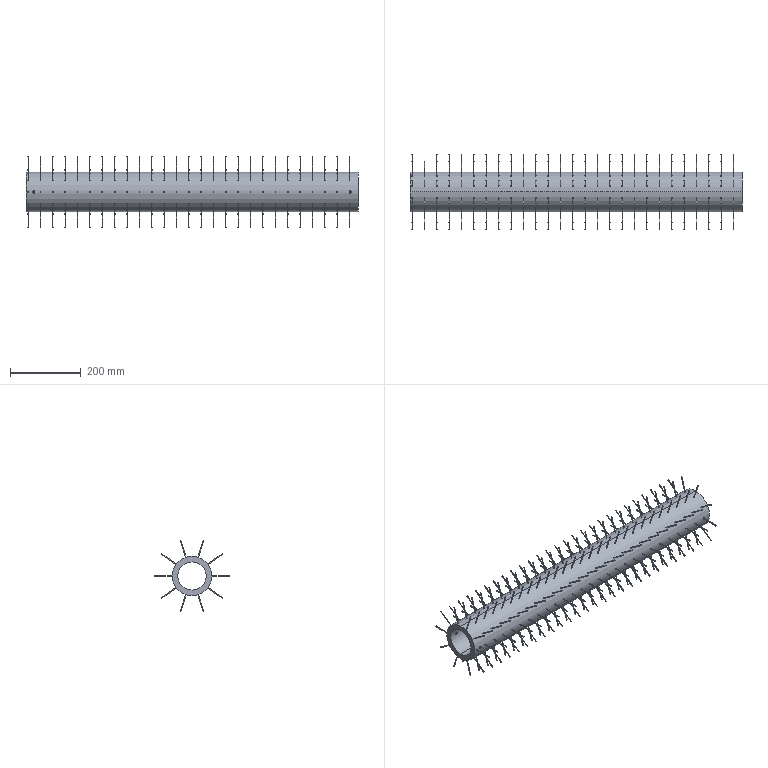Part | NX | features BREP 270 | 270 solids | 1090 faces | box 940 x 212 x 202.242 mm | volume 4576402 mm3 | cylinder 550 | plane 540 | commonest cylinder face diameters 2 x538 6 x8 80 x2 112 x2